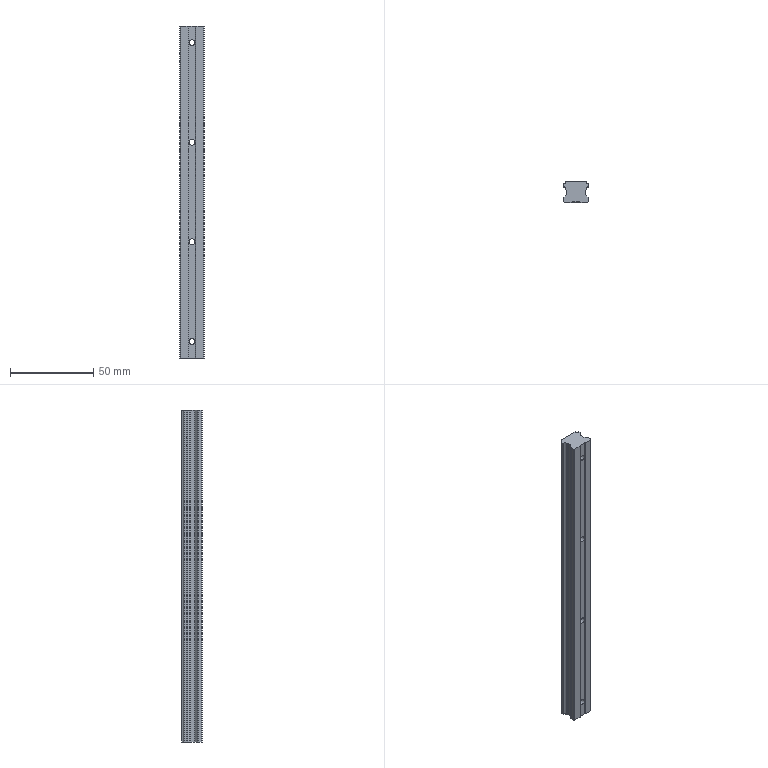Part | STEP file | transport section slide rail EG15_RAIL | 1 solid | 58 faces | box 15 x 12.5 x 200 mm | volume 31877 mm3 | cylinder 34 | plane 24 | commonest cylinder face diameters 0.6 x11 6 x8 3.5 x6 3 x5 1 x2 3.4 x2